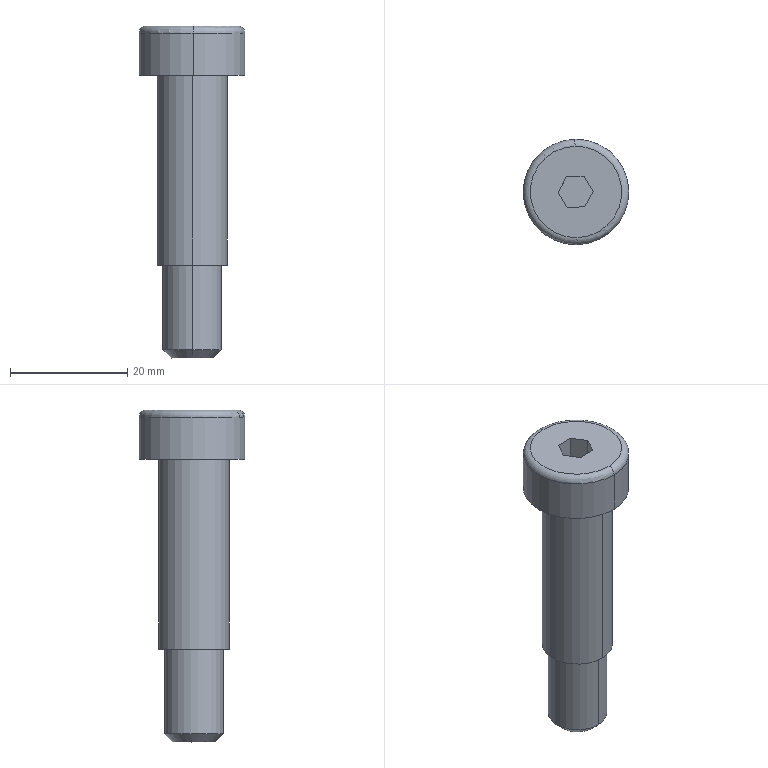Part | SolidWorks | features BaseBody 1 | 1 solid | 21 faces | box 18.001 x 18 x 56.624 mm | volume 6859 mm3 | plane 11 | cylinder 6 | torus 2 | cone 2 | commonest cylinder face diameters 10 x2 12 x2 18 x2
STEP:
#1=CARTESIAN_POINT('',(377.104,200.564,27.671));
#2=VERTEX_POINT('',#1);
#3=CARTESIAN_POINT('',(377.483,182.568,27.671));
#4=VERTEX_POINT('',#3);
#5=CARTESIAN_POINT('',(377.294,191.566,27.671));
#6=DIRECTION('',(-0.0001435,-0.000000521,1.));
#7=DIRECTION('',(0.02104,-0.9998,0.000002497));
#8=AXIS2_PLACEMENT_3D('',#5,#6,#7);
#9=CIRCLE('',#8,9.);
#10=EDGE_CURVE('',#2,#4,#9,.T.);
#11=ORIENTED_EDGE('',*,*,#10,.T.);
#12=CARTESIAN_POINT('',(377.458,183.768,28.871));
#13=VERTEX_POINT('',#12);
#14=CARTESIAN_POINT('',(377.458,183.768,27.671));
#15=DIRECTION('',(-0.9998,-0.02104,-0.0001435));
#16=DIRECTION('',(0.02104,-0.9998,0.));
#17=AXIS2_PLACEMENT_3D('',#14,#15,#16);
#18=CIRCLE('',#17,1.2);
#19=EDGE_CURVE('',#4,#13,#18,.T.);
#20=ORIENTED_EDGE('',*,*,#19,.T.);
#21=CARTESIAN_POINT('',(377.129,199.364,28.871));
#22=VERTEX_POINT('',#21);
#23=CARTESIAN_POINT('',(377.294,191.566,28.871));
#24=DIRECTION('',(-0.0001435,-0.000000521,1.));
#25=DIRECTION('',(0.02104,-0.9998,0.000002497));
#26=AXIS2_PLACEMENT_3D('',#23,#24,#25);
#27=CIRCLE('',#26,7.8);
#28=EDGE_CURVE('',#22,#13,#27,.T.);
#29=ORIENTED_EDGE('',*,*,#28,.F.);
#30=CARTESIAN_POINT('',(377.13,199.364,27.671));
#31=DIRECTION('',(0.9998,0.02104,0.0001435));
#32=DIRECTION('',(-0.02104,0.9998,0.));
#33=AXIS2_PLACEMENT_3D('',#30,#31,#32);
#34=CIRCLE('',#33,1.2);
#35=EDGE_CURVE('',#2,#22,#34,.T.);
#36=ORIENTED_EDGE('',*,*,#35,.F.);
#37=EDGE_LOOP('',(#11,#20,#29,#36));
#38=FACE_OUTER_BOUND('',#37,.T.);
#39=CARTESIAN_POINT('',(377.294,191.566,27.671));
#40=DIRECTION('',(-0.0001435,-0.000000521,1.));
#41=DIRECTION('',(-0.02104,0.9998,-0.000002497));
#42=AXIS2_PLACEMENT_3D('',#39,#40,#41);
#43=TOROIDAL_SURFACE('',#42,7.8,1.2);
#44=ADVANCED_FACE('',(#38),#43,.T.);
#45=CARTESIAN_POINT('',(377.484,182.568,20.471));
#46=VERTEX_POINT('',#45);
#47=CARTESIAN_POINT('',(377.105,200.564,20.471));
#48=VERTEX_POINT('',#47);
#49=CARTESIAN_POINT('',(377.295,191.566,20.471));
#50=DIRECTION('',(0.0001435,0.000000521,-1.));
#51=DIRECTION('',(-0.02104,0.9998,-0.000002497));
#52=AXIS2_PLACEMENT_3D('',#49,#50,#51);
#53=CIRCLE('',#52,9.);
#54=EDGE_CURVE('',#46,#48,#53,.T.);
#55=ORIENTED_EDGE('',*,*,#54,.F.);
#56=CARTESIAN_POINT('',(377.484,182.568,20.471));
#57=DIRECTION('',(-0.0001435,-0.000000521,1.));
#58=VECTOR('',#57,1000.);
#59=LINE('',#56,#58);
#60=EDGE_CURVE('',#46,#4,#59,.T.);
#61=ORIENTED_EDGE('',*,*,#60,.T.);
#62=ORIENTED_EDGE('',*,*,#10,.F.);
#63=CARTESIAN_POINT('',(377.105,200.564,20.471));
#64=DIRECTION('',(-0.0001435,-0.000000521,1.));
#65=VECTOR('',#64,1000.);
#66=LINE('',#63,#65);
#67=EDGE_CURVE('',#48,#2,#66,.T.);
#68=ORIENTED_EDGE('',*,*,#67,.F.);
#69=EDGE_LOOP('',(#55,#61,#62,#68));
#70=FACE_OUTER_BOUND('',#69,.T.);
#71=CARTESIAN_POINT('',(377.295,191.566,20.471));
#72=DIRECTION('',(-0.0001435,-0.000000521,1.));
#73=DIRECTION('',(-0.02104,0.9998,-0.000002497));
#74=AXIS2_PLACEMENT_3D('',#71,#72,#73);
#75=CYLINDRICAL_SURFACE('',#74,9.);
#76=ADVANCED_FACE('',(#70),#75,.T.);
#77=CARTESIAN_POINT('',(377.179,197.227,20.471));
#78=VERTEX_POINT('',#77);
#79=CARTESIAN_POINT('',(377.431,185.23,20.471));
#80=VERTEX_POINT('',#79);
#81=CARTESIAN_POINT('',(377.305,191.228,20.471));
#82=DIRECTION('',(-0.0001435,-0.000000521,1.));
#83=DIRECTION('',(0.02104,-0.9998,0.000002497));
#84=AXIS2_PLACEMENT_3D('',#81,#82,#83);
#85=CIRCLE('',#84,6.);
#86=EDGE_CURVE('',#78,#80,#85,.T.);
#87=ORIENTED_EDGE('',*,*,#86,.F.);
#88=CARTESIAN_POINT('',(377.183,197.227,-11.912));
#89=VERTEX_POINT('',#88);
#90=CARTESIAN_POINT('',(377.183,197.227,-11.726));
#91=DIRECTION('',(0.0001435,0.000000521,-1.));
#92=VECTOR('',#91,1000.);
#93=LINE('',#90,#92);
#94=EDGE_CURVE('',#78,#89,#93,.T.);
#95=ORIENTED_EDGE('',*,*,#94,.T.);
#96=CARTESIAN_POINT('',(377.436,185.23,-11.911));
#97=VERTEX_POINT('',#96);
#98=CARTESIAN_POINT('',(377.31,191.228,-11.911));
#99=DIRECTION('',(0.0001435,0.000000521,-1.));
#100=DIRECTION('',(-1.,0.,-0.0001435));
#101=AXIS2_PLACEMENT_3D('',#98,#99,#100);
#102=CIRCLE('',#101,6.);
#103=EDGE_CURVE('',#97,#89,#102,.T.);
#104=ORIENTED_EDGE('',*,*,#103,.F.);
#105=CARTESIAN_POINT('',(377.436,185.23,-11.726));
#106=DIRECTION('',(0.0001435,0.000000521,-1.));
#107=VECTOR('',#106,1000.);
#108=LINE('',#105,#107);
#109=EDGE_CURVE('',#80,#97,#108,.T.);
#110=ORIENTED_EDGE('',*,*,#109,.F.);
#111=EDGE_LOOP('',(#87,#95,#104,#110));
#112=FACE_OUTER_BOUND('',#111,.T.);
#113=CARTESIAN_POINT('',(377.309,191.228,-11.726));
#114=DIRECTION('',(0.0001435,0.000000521,-1.));
#115=DIRECTION('',(0.02104,-0.9998,0.000002497));
#116=AXIS2_PLACEMENT_3D('',#113,#114,#115);
#117=CYLINDRICAL_SURFACE('',#116,6.);
#118=ADVANCED_FACE('',(#112),#117,.T.);
#119=CARTESIAN_POINT('',(377.207,196.227,-11.912));
#120=VERTEX_POINT('',#119);
#121=CARTESIAN_POINT('',(377.417,186.23,-11.911));
#122=VERTEX_POINT('',#121);
#123=CARTESIAN_POINT('',(377.312,191.228,-11.911));
#124=DIRECTION('',(-0.0001435,-0.000000521,1.));
#125=DIRECTION('',(0.02104,-0.9998,0.000002497));
#126=AXIS2_PLACEMENT_3D('',#123,#124,#125);
#127=CIRCLE('',#126,5.);
#128=EDGE_CURVE('',#120,#122,#127,.T.);
#129=ORIENTED_EDGE('',*,*,#128,.F.);
#130=CARTESIAN_POINT('',(377.209,196.227,-26.352));
#131=VERTEX_POINT('',#130);
#132=CARTESIAN_POINT('',(377.207,196.227,-14.312));
#133=DIRECTION('',(0.0001435,0.000000521,-1.));
#134=VECTOR('',#133,1000.);
#135=LINE('',#132,#134);
#136=EDGE_CURVE('',#120,#131,#135,.T.);
#137=ORIENTED_EDGE('',*,*,#136,.T.);
#138=CARTESIAN_POINT('',(377.419,186.23,-26.351));
#139=VERTEX_POINT('',#138);
#140=CARTESIAN_POINT('',(377.314,191.228,-26.351));
#141=DIRECTION('',(0.0001435,0.000000521,-1.));
#142=DIRECTION('',(0.02104,-0.9998,0.000002497));
#143=AXIS2_PLACEMENT_3D('',#140,#141,#142);
#144=CIRCLE('',#143,5.);
#145=EDGE_CURVE('',#139,#131,#144,.T.);
#146=ORIENTED_EDGE('',*,*,#145,.F.);
#147=CARTESIAN_POINT('',(377.418,186.23,-14.311));
#148=DIRECTION('',(0.0001435,0.000000521,-1.));
#149=VECTOR('',#148,1000.);
#150=LINE('',#147,#149);
#151=EDGE_CURVE('',#122,#139,#150,.T.);
#152=ORIENTED_EDGE('',*,*,#151,.F.);
#153=EDGE_LOOP('',(#129,#137,#146,#152));
#154=FACE_OUTER_BOUND('',#153,.T.);
#155=CARTESIAN_POINT('',(377.312,191.228,-14.311));
#156=DIRECTION('',(0.0001435,0.000000521,-1.));
#157=DIRECTION('',(0.02104,-0.9998,0.000002497));
#158=AXIS2_PLACEMENT_3D('',#155,#156,#157);
#159=CYLINDRICAL_SURFACE('',#158,5.);
#160=ADVANCED_FACE('',(#154),#159,.T.);
#161=CARTESIAN_POINT('',(377.39,187.629,-27.751));
#162=VERTEX_POINT('',#161);
#163=CARTESIAN_POINT('',(377.239,194.828,-27.751));
#164=VERTEX_POINT('',#163);
#165=CARTESIAN_POINT('',(377.314,191.228,-27.751));
#166=DIRECTION('',(0.0001435,0.000000521,-1.));
#167=DIRECTION('',(0.02104,-0.9998,0.000002497));
#168=AXIS2_PLACEMENT_3D('',#165,#166,#167);
#169=CIRCLE('',#168,3.6);
#170=EDGE_CURVE('',#162,#164,#169,.T.);
#171=ORIENTED_EDGE('',*,*,#170,.F.);
#172=CARTESIAN_POINT('',(377.405,186.929,-27.051));
#173=DIRECTION('',(0.01477,-0.707,0.7071));
#174=VECTOR('',#173,1000.);
#175=LINE('',#172,#174);
#176=EDGE_CURVE('',#162,#139,#175,.T.);
#177=ORIENTED_EDGE('',*,*,#176,.T.);
#178=ORIENTED_EDGE('',*,*,#145,.T.);
#179=CARTESIAN_POINT('',(377.224,195.528,-27.052));
#180=DIRECTION('',(-0.01498,0.7069,0.7071));
#181=VECTOR('',#180,1000.);
#182=LINE('',#179,#181);
#183=EDGE_CURVE('',#164,#131,#182,.T.);
#184=ORIENTED_EDGE('',*,*,#183,.F.);
#185=EDGE_LOOP('',(#171,#177,#178,#184));
#186=FACE_OUTER_BOUND('',#185,.T.);
#187=CARTESIAN_POINT('',(377.314,191.228,-27.051));
#188=DIRECTION('',(-0.0001435,-0.000000521,1.));
#189=DIRECTION('',(-0.02104,0.9998,-0.000002497));
#190=AXIS2_PLACEMENT_3D('',#187,#188,#189);
#191=CONICAL_SURFACE('',#190,4.3,0.7854);
#192=ADVANCED_FACE('',(#186),#191,.T.);
#193=CARTESIAN_POINT('',(377.314,191.228,-27.751));
#194=DIRECTION('',(0.0001435,0.000000521,-1.));
#195=DIRECTION('',(0.02104,-0.9998,0.000002497));
#196=AXIS2_PLACEMENT_3D('',#193,#194,#195);
#197=CIRCLE('',#196,3.6);
#198=EDGE_CURVE('',#164,#162,#197,.T.);
#199=ORIENTED_EDGE('',*,*,#198,.T.);
#200=ORIENTED_EDGE('',*,*,#170,.T.);
#201=EDGE_LOOP('',(#199,#200));
#202=FACE_OUTER_BOUND('',#201,.T.);
#203=CARTESIAN_POINT('',(377.314,191.228,-27.751));
#204=DIRECTION('',(0.0001435,0.000000521,-1.));
#205=DIRECTION('',(0.,-1.,-0.000000521));
#206=AXIS2_PLACEMENT_3D('',#203,#204,#205);
#207=PLANE('',#206);
#208=ADVANCED_FACE('',(#202),#207,.T.);
#209=ORIENTED_EDGE('',*,*,#176,.F.);
#210=ORIENTED_EDGE('',*,*,#198,.F.);
#211=ORIENTED_EDGE('',*,*,#183,.T.);
#212=CARTESIAN_POINT('',(377.314,191.228,-26.351));
#213=DIRECTION('',(0.0001435,0.000000521,-1.));
#214=DIRECTION('',(0.02104,-0.9998,0.000002497));
#215=AXIS2_PLACEMENT_3D('',#212,#213,#214);
#216=CIRCLE('',#215,5.);
#217=EDGE_CURVE('',#131,#139,#216,.T.);
#218=ORIENTED_EDGE('',*,*,#217,.T.);
#219=EDGE_LOOP('',(#209,#210,#211,#218));
#220=FACE_OUTER_BOUND('',#219,.T.);
#221=CARTESIAN_POINT('',(377.314,191.228,-27.051));
#222=DIRECTION('',(-0.0001435,-0.000000521,1.));
#223=DIRECTION('',(-0.02104,0.9998,-0.000002497));
#224=AXIS2_PLACEMENT_3D('',#221,#222,#223);
#225=CONICAL_SURFACE('',#224,4.3,0.7854);
#226=ADVANCED_FACE('',(#220),#225,.T.);
#227=ORIENTED_EDGE('',*,*,#136,.F.);
#228=CARTESIAN_POINT('',(377.312,191.228,-11.911));
#229=DIRECTION('',(-0.0001435,-0.000000521,1.));
#230=DIRECTION('',(0.02104,-0.9998,0.000002497));
#231=AXIS2_PLACEMENT_3D('',#228,#229,#230);
#232=CIRCLE('',#231,5.);
#233=EDGE_CURVE('',#122,#120,#232,.T.);
#234=ORIENTED_EDGE('',*,*,#233,.F.);
#235=ORIENTED_EDGE('',*,*,#151,.T.);
#236=ORIENTED_EDGE('',*,*,#217,.F.);
#237=EDGE_LOOP('',(#227,#234,#235,#236));
#238=FACE_OUTER_BOUND('',#237,.T.);
#239=CARTESIAN_POINT('',(377.312,191.228,-14.311));
#240=DIRECTION('',(0.0001435,0.000000521,-1.));
#241=DIRECTION('',(0.02104,-0.9998,0.000002497));
#242=AXIS2_PLACEMENT_3D('',#239,#240,#241);
#243=CYLINDRICAL_SURFACE('',#242,5.);
#244=ADVANCED_FACE('',(#238),#243,.T.);
#245=ORIENTED_EDGE('',*,*,#233,.T.);
#246=ORIENTED_EDGE('',*,*,#128,.T.);
#247=EDGE_LOOP('',(#245,#246));
#248=FACE_BOUND('',#247,.T.);
#249=ORIENTED_EDGE('',*,*,#103,.T.);
#250=CARTESIAN_POINT('',(377.31,191.228,-11.911));
#251=DIRECTION('',(0.0001435,0.000000521,-1.));
#252=DIRECTION('',(-1.,0.,-0.0001435));
#253=AXIS2_PLACEMENT_3D('',#250,#251,#252);
#254=CIRCLE('',#253,6.);
#255=EDGE_CURVE('',#89,#97,#254,.T.);
#256=ORIENTED_EDGE('',*,*,#255,.T.);
#257=EDGE_LOOP('',(#249,#256));
#258=FACE_OUTER_BOUND('',#257,.T.);
#259=CARTESIAN_POINT('',(377.312,191.228,-11.911));
#260=DIRECTION('',(0.0001435,0.000000521,-1.));
#261=DIRECTION('',(0.,-1.,-0.000000521));
#262=AXIS2_PLACEMENT_3D('',#259,#260,#261);
#263=PLANE('',#262);
#264=ADVANCED_FACE('',(#248,#258),#263,.T.);
#265=ORIENTED_EDGE('',*,*,#94,.F.);
#266=CARTESIAN_POINT('',(377.305,191.228,20.471));
#267=DIRECTION('',(-0.0001435,-0.000000521,1.));
#268=DIRECTION('',(0.02104,-0.9998,0.000002497));
#269=AXIS2_PLACEMENT_3D('',#266,#267,#268);
#270=CIRCLE('',#269,6.);
#271=EDGE_CURVE('',#80,#78,#270,.T.);
#272=ORIENTED_EDGE('',*,*,#271,.F.);
#273=ORIENTED_EDGE('',*,*,#109,.T.);
#274=ORIENTED_EDGE('',*,*,#255,.F.);
#275=EDGE_LOOP('',(#265,#272,#273,#274));
#276=FACE_OUTER_BOUND('',#275,.T.);
#277=CARTESIAN_POINT('',(377.309,191.228,-11.726));
#278=DIRECTION('',(0.0001435,0.000000521,-1.));
#279=DIRECTION('',(0.02104,-0.9998,0.000002497));
#280=AXIS2_PLACEMENT_3D('',#277,#278,#279);
#281=CYLINDRICAL_SURFACE('',#280,6.);
#282=ADVANCED_FACE('',(#276),#281,.T.);
#283=ORIENTED_EDGE('',*,*,#271,.T.);
#284=ORIENTED_EDGE('',*,*,#86,.T.);
#285=EDGE_LOOP('',(#283,#284));
#286=FACE_BOUND('',#285,.T.);
#287=CARTESIAN_POINT('',(377.295,191.566,20.471));
#288=DIRECTION('',(0.0001435,0.000000521,-1.));
#289=DIRECTION('',(-0.02104,0.9998,-0.000002497));
#290=AXIS2_PLACEMENT_3D('',#287,#288,#289);
#291=CIRCLE('',#290,9.);
#292=EDGE_CURVE('',#48,#46,#291,.T.);
#293=ORIENTED_EDGE('',*,*,#292,.T.);
#294=ORIENTED_EDGE('',*,*,#54,.T.);
#295=EDGE_LOOP('',(#293,#294));
#296=FACE_OUTER_BOUND('',#295,.T.);
#297=CARTESIAN_POINT('',(377.295,191.566,20.471));
#298=DIRECTION('',(0.0001435,0.000000521,-1.));
#299=DIRECTION('',(0.,-1.,-0.000000521));
#300=AXIS2_PLACEMENT_3D('',#297,#298,#299);
#301=PLANE('',#300);
#302=ADVANCED_FACE('',(#286,#296),#301,.T.);
#303=ORIENTED_EDGE('',*,*,#60,.F.);
#304=ORIENTED_EDGE('',*,*,#292,.F.);
#305=ORIENTED_EDGE('',*,*,#67,.T.);
#306=CARTESIAN_POINT('',(377.294,191.566,27.671));
#307=DIRECTION('',(-0.0001435,-0.000000521,1.));
#308=DIRECTION('',(0.02104,-0.9998,0.000002497));
#309=AXIS2_PLACEMENT_3D('',#306,#307,#308);
#310=CIRCLE('',#309,9.);
#311=EDGE_CURVE('',#4,#2,#310,.T.);
#312=ORIENTED_EDGE('',*,*,#311,.F.);
#313=EDGE_LOOP('',(#303,#304,#305,#312));
#314=FACE_OUTER_BOUND('',#313,.T.);
#315=CARTESIAN_POINT('',(377.295,191.566,20.471));
#316=DIRECTION('',(-0.0001435,-0.000000521,1.));
#317=DIRECTION('',(-0.02104,0.9998,-0.000002497));
#318=AXIS2_PLACEMENT_3D('',#315,#316,#317);
#319=CYLINDRICAL_SURFACE('',#318,9.);
#320=ADVANCED_FACE('',(#314),#319,.T.);
#321=ORIENTED_EDGE('',*,*,#19,.F.);
#322=ORIENTED_EDGE('',*,*,#311,.T.);
#323=ORIENTED_EDGE('',*,*,#35,.T.);
#324=CARTESIAN_POINT('',(377.294,191.566,28.871));
#325=DIRECTION('',(-0.0001435,-0.000000521,1.));
#326=DIRECTION('',(0.02104,-0.9998,0.000002497));
#327=AXIS2_PLACEMENT_3D('',#324,#325,#326);
#328=CIRCLE('',#327,7.8);
#329=EDGE_CURVE('',#13,#22,#328,.T.);
#330=ORIENTED_EDGE('',*,*,#329,.F.);
#331=EDGE_LOOP('',(#321,#322,#323,#330));
#332=FACE_OUTER_BOUND('',#331,.T.);
#333=CARTESIAN_POINT('',(377.294,191.566,27.671));
#334=DIRECTION('',(-0.0001435,-0.000000521,1.));
#335=DIRECTION('',(-0.02104,0.9998,-0.000002497));
#336=AXIS2_PLACEMENT_3D('',#333,#334,#335);
#337=TOROIDAL_SURFACE('',#336,7.8,1.2);
#338=ADVANCED_FACE('',(#332),#337,.T.);
#339=CARTESIAN_POINT('',(375.792,188.955,22.871));
#340=VERTEX_POINT('',#339);
#341=CARTESIAN_POINT('',(378.792,189.018,22.871));
#342=VERTEX_POINT('',#341);
#343=CARTESIAN_POINT('',(375.792,188.955,22.871));
#344=DIRECTION('',(0.9998,0.02104,0.0001435));
#345=VECTOR('',#344,1000.);
#346=LINE('',#343,#345);
#347=EDGE_CURVE('',#340,#342,#346,.T.);
#348=ORIENTED_EDGE('',*,*,#347,.T.);
#349=CARTESIAN_POINT('',(380.237,191.648,22.871));
#350=VERTEX_POINT('',#349);
#351=CARTESIAN_POINT('',(378.792,189.018,22.871));
#352=DIRECTION('',(0.4817,0.8764,0.00006956));
#353=VECTOR('',#352,1000.);
#354=LINE('',#351,#353);
#355=EDGE_CURVE('',#342,#350,#354,.T.);
#356=ORIENTED_EDGE('',*,*,#355,.T.);
#357=CARTESIAN_POINT('',(378.682,194.213,22.871));
#358=VERTEX_POINT('',#357);
#359=CARTESIAN_POINT('',(380.237,191.648,22.871));
#360=DIRECTION('',(-0.5181,0.8553,-0.00007389));
#361=VECTOR('',#360,1000.);
#362=LINE('',#359,#361);
#363=EDGE_CURVE('',#350,#358,#362,.T.);
#364=ORIENTED_EDGE('',*,*,#363,.T.);
#365=CARTESIAN_POINT('',(375.683,194.15,22.871));
#366=VERTEX_POINT('',#365);
#367=CARTESIAN_POINT('',(378.682,194.213,22.871));
#368=DIRECTION('',(-0.9998,-0.02104,-0.0001435));
#369=VECTOR('',#368,1000.);
#370=LINE('',#367,#369);
#371=EDGE_CURVE('',#358,#366,#370,.T.);
#372=ORIENTED_EDGE('',*,*,#371,.T.);
#373=CARTESIAN_POINT('',(374.238,191.521,22.87));
#374=VERTEX_POINT('',#373);
#375=CARTESIAN_POINT('',(375.683,194.15,22.871));
#376=DIRECTION('',(-0.4817,-0.8764,-0.00006956));
#377=VECTOR('',#376,1000.);
#378=LINE('',#375,#377);
#379=EDGE_CURVE('',#366,#374,#378,.T.);
#380=ORIENTED_EDGE('',*,*,#379,.T.);
#381=CARTESIAN_POINT('',(374.238,191.521,22.87));
#382=DIRECTION('',(0.5181,-0.8553,0.00007389));
#383=VECTOR('',#382,1000.);
#384=LINE('',#381,#383);
#385=EDGE_CURVE('',#374,#340,#384,.T.);
#386=ORIENTED_EDGE('',*,*,#385,.T.);
#387=EDGE_LOOP('',(#348,#356,#364,#372,#380,#386));
#388=FACE_OUTER_BOUND('',#387,.T.);
#389=CARTESIAN_POINT('',(376.682,220.659,22.871));
#390=DIRECTION('',(-0.0001435,-0.000000521,1.));
#391=DIRECTION('',(-0.003633,1.,0.));
#392=AXIS2_PLACEMENT_3D('',#389,#390,#391);
#393=PLANE('',#392);
#394=ADVANCED_FACE('',(#388),#393,.T.);
#395=CARTESIAN_POINT('',(378.791,189.018,28.871));
#396=VERTEX_POINT('',#395);
#397=CARTESIAN_POINT('',(378.791,189.018,28.871));
#398=DIRECTION('',(0.0001435,0.000000521,-1.));
#399=VECTOR('',#398,1000.);
#400=LINE('',#397,#399);
#401=EDGE_CURVE('',#396,#342,#400,.T.);
#402=ORIENTED_EDGE('',*,*,#401,.T.);
#403=ORIENTED_EDGE('',*,*,#347,.F.);
#404=CARTESIAN_POINT('',(375.791,188.955,28.871));
#405=VERTEX_POINT('',#404);
#406=CARTESIAN_POINT('',(375.791,188.955,28.871));
#407=DIRECTION('',(0.0001435,0.000000521,-1.));
#408=VECTOR('',#407,1000.);
#409=LINE('',#406,#408);
#410=EDGE_CURVE('',#405,#340,#409,.T.);
#411=ORIENTED_EDGE('',*,*,#410,.F.);
#412=CARTESIAN_POINT('',(378.791,189.018,28.871));
#413=DIRECTION('',(-0.9998,-0.02104,-0.0001435));
#414=VECTOR('',#413,1000.);
#415=LINE('',#412,#414);
#416=EDGE_CURVE('',#396,#405,#415,.T.);
#417=ORIENTED_EDGE('',*,*,#416,.F.);
#418=EDGE_LOOP('',(#402,#403,#411,#417));
#419=FACE_OUTER_BOUND('',#418,.T.);
#420=CARTESIAN_POINT('',(378.792,189.018,22.871));
#421=DIRECTION('',(0.02104,-0.9998,0.000002497));
#422=DIRECTION('',(0.,-0.000002498,-1.));
#423=AXIS2_PLACEMENT_3D('',#420,#421,#422);
#424=PLANE('',#423);
#425=ADVANCED_FACE('',(#419),#424,.F.);
#426=CARTESIAN_POINT('',(380.236,191.648,28.871));
#427=VERTEX_POINT('',#426);
#428=CARTESIAN_POINT('',(380.236,191.648,28.871));
#429=DIRECTION('',(0.0001435,0.000000521,-1.));
#430=VECTOR('',#429,1000.);
#431=LINE('',#428,#430);
#432=EDGE_CURVE('',#427,#350,#431,.T.);
#433=ORIENTED_EDGE('',*,*,#432,.T.);
#434=ORIENTED_EDGE('',*,*,#355,.F.);
#435=ORIENTED_EDGE('',*,*,#401,.F.);
#436=CARTESIAN_POINT('',(380.236,191.648,28.871));
#437=DIRECTION('',(-0.4817,-0.8764,-0.00006956));
#438=VECTOR('',#437,1000.);
#439=LINE('',#436,#438);
#440=EDGE_CURVE('',#427,#396,#439,.T.);
#441=ORIENTED_EDGE('',*,*,#440,.F.);
#442=EDGE_LOOP('',(#433,#434,#435,#441));
#443=FACE_OUTER_BOUND('',#442,.T.);
#444=CARTESIAN_POINT('',(380.237,191.648,22.871));
#445=DIRECTION('',(0.8764,-0.4817,0.0001255));
#446=DIRECTION('',(0.,-0.0002605,-1.));
#447=AXIS2_PLACEMENT_3D('',#444,#445,#446);
#448=PLANE('',#447);
#449=ADVANCED_FACE('',(#443),#448,.F.);
#450=CARTESIAN_POINT('',(378.681,194.213,28.871));
#451=VERTEX_POINT('',#450);
#452=CARTESIAN_POINT('',(378.681,194.213,28.871));
#453=DIRECTION('',(0.0001435,0.000000521,-1.));
#454=VECTOR('',#453,1000.);
#455=LINE('',#452,#454);
#456=EDGE_CURVE('',#451,#358,#455,.T.);
#457=ORIENTED_EDGE('',*,*,#456,.T.);
#458=ORIENTED_EDGE('',*,*,#363,.F.);
#459=ORIENTED_EDGE('',*,*,#432,.F.);
#460=CARTESIAN_POINT('',(378.681,194.213,28.871));
#461=DIRECTION('',(0.5181,-0.8553,0.00007389));
#462=VECTOR('',#461,1000.);
#463=LINE('',#460,#462);
#464=EDGE_CURVE('',#451,#427,#463,.T.);
#465=ORIENTED_EDGE('',*,*,#464,.F.);
#466=EDGE_LOOP('',(#457,#458,#459,#465));
#467=FACE_OUTER_BOUND('',#466,.T.);
#468=CARTESIAN_POINT('',(378.682,194.213,22.871));
#469=DIRECTION('',(0.8553,0.5181,0.000123));
#470=DIRECTION('',(0.,0.0002374,-1.));
#471=AXIS2_PLACEMENT_3D('',#468,#469,#470);
#472=PLANE('',#471);
#473=ADVANCED_FACE('',(#467),#472,.F.);
#474=CARTESIAN_POINT('',(375.682,194.15,28.871));
#475=VERTEX_POINT('',#474);
#476=CARTESIAN_POINT('',(375.682,194.15,28.871));
#477=DIRECTION('',(0.0001435,0.000000521,-1.));
#478=VECTOR('',#477,1000.);
#479=LINE('',#476,#478);
#480=EDGE_CURVE('',#475,#366,#479,.T.);
#481=ORIENTED_EDGE('',*,*,#480,.T.);
#482=ORIENTED_EDGE('',*,*,#371,.F.);
#483=ORIENTED_EDGE('',*,*,#456,.F.);
#484=CARTESIAN_POINT('',(375.682,194.15,28.871));
#485=DIRECTION('',(0.9998,0.02104,0.0001435));
#486=VECTOR('',#485,1000.);
#487=LINE('',#484,#486);
#488=EDGE_CURVE('',#475,#451,#487,.T.);
#489=ORIENTED_EDGE('',*,*,#488,.F.);
#490=EDGE_LOOP('',(#481,#482,#483,#489));
#491=FACE_OUTER_BOUND('',#490,.T.);
#492=CARTESIAN_POINT('',(375.683,194.15,22.871));
#493=DIRECTION('',(-0.02104,0.9998,-0.000002497));
#494=DIRECTION('',(-0.0001187,0.,1.));
#495=AXIS2_PLACEMENT_3D('',#492,#493,#494);
#496=PLANE('',#495);
#497=ADVANCED_FACE('',(#491),#496,.F.);
#498=CARTESIAN_POINT('',(374.237,191.521,28.87));
#499=VERTEX_POINT('',#498);
#500=CARTESIAN_POINT('',(374.237,191.521,28.87));
#501=DIRECTION('',(0.0001435,0.000000521,-1.));
#502=VECTOR('',#501,1000.);
#503=LINE('',#500,#502);
#504=EDGE_CURVE('',#499,#374,#503,.T.);
#505=ORIENTED_EDGE('',*,*,#504,.T.);
#506=ORIENTED_EDGE('',*,*,#379,.F.);
#507=ORIENTED_EDGE('',*,*,#480,.F.);
#508=CARTESIAN_POINT('',(374.237,191.521,28.87));
#509=DIRECTION('',(0.4817,0.8764,0.00006956));
#510=VECTOR('',#509,1000.);
#511=LINE('',#508,#510);
#512=EDGE_CURVE('',#499,#475,#511,.T.);
#513=ORIENTED_EDGE('',*,*,#512,.F.);
#514=EDGE_LOOP('',(#505,#506,#507,#513));
#515=FACE_OUTER_BOUND('',#514,.T.);
#516=CARTESIAN_POINT('',(374.238,191.521,22.87));
#517=DIRECTION('',(-0.8764,0.4817,-0.0001255));
#518=DIRECTION('',(-0.0001432,0.,1.));
#519=AXIS2_PLACEMENT_3D('',#516,#517,#518);
#520=PLANE('',#519);
#521=ADVANCED_FACE('',(#515),#520,.F.);
#522=ORIENTED_EDGE('',*,*,#410,.T.);
#523=ORIENTED_EDGE('',*,*,#385,.F.);
#524=ORIENTED_EDGE('',*,*,#504,.F.);
#525=CARTESIAN_POINT('',(375.791,188.955,28.871));
#526=DIRECTION('',(-0.5181,0.8553,-0.00007389));
#527=VECTOR('',#526,1000.);
#528=LINE('',#525,#527);
#529=EDGE_CURVE('',#405,#499,#528,.T.);
#530=ORIENTED_EDGE('',*,*,#529,.F.);
#531=EDGE_LOOP('',(#522,#523,#524,#530));
#532=FACE_OUTER_BOUND('',#531,.T.);
#533=CARTESIAN_POINT('',(375.792,188.955,22.871));
#534=DIRECTION('',(-0.8553,-0.5181,-0.000123));
#535=DIRECTION('',(-0.5181,0.8553,0.));
#536=AXIS2_PLACEMENT_3D('',#533,#534,#535);
#537=PLANE('',#536);
#538=ADVANCED_FACE('',(#532),#537,.F.);
#539=ORIENTED_EDGE('',*,*,#512,.T.);
#540=ORIENTED_EDGE('',*,*,#488,.T.);
#541=ORIENTED_EDGE('',*,*,#464,.T.);
#542=ORIENTED_EDGE('',*,*,#440,.T.);
#543=ORIENTED_EDGE('',*,*,#416,.T.);
#544=ORIENTED_EDGE('',*,*,#529,.T.);
#545=EDGE_LOOP('',(#539,#540,#541,#542,#543,#544));
#546=FACE_BOUND('',#545,.T.);
#547=ORIENTED_EDGE('',*,*,#28,.T.);
#548=ORIENTED_EDGE('',*,*,#329,.T.);
#549=EDGE_LOOP('',(#547,#548));
#550=FACE_OUTER_BOUND('',#549,.T.);
#551=CARTESIAN_POINT('',(377.294,191.566,28.871));
#552=DIRECTION('',(-0.0001435,-0.000000521,1.));
#553=DIRECTION('',(-0.003633,1.,0.));
#554=AXIS2_PLACEMENT_3D('',#551,#552,#553);
#555=PLANE('',#554);
#556=ADVANCED_FACE('',(#546,#550),#555,.T.);
#557=CLOSED_SHELL('',(#44,#76,#118,#160,#192,#208,#226,#244,#264,#282,#302,#320,#338,#394,#425,#449,#473,#497,#521,#538,#556));
#558=MANIFOLD_SOLID_BREP('',#557);
#559=CARTESIAN_POINT('',(0.,0.,0.));
#560=DIRECTION('',(0.,0.,1.));
#561=DIRECTION('',(1.,0.,0.));
#562=AXIS2_PLACEMENT_3D('',#559,#560,#561);
#563=(LENGTH_UNIT()NAMED_UNIT(*)SI_UNIT(.MILLI.,.METRE.));
#564=UNCERTAINTY_MEASURE_WITH_UNIT(LENGTH_MEASURE(0.00001),#563,'','');
#565=(NAMED_UNIT(*)PLANE_ANGLE_UNIT()SI_UNIT($,.RADIAN.));
#566=(NAMED_UNIT(*)SI_UNIT($,.STERADIAN.)SOLID_ANGLE_UNIT());
#567=(GEOMETRIC_REPRESENTATION_CONTEXT(3)GLOBAL_UNCERTAINTY_ASSIGNED_CONTEXT((#564))GLOBAL_UNIT_ASSIGNED_CONTEXT((#563,#565,#566))REPRESENTATION_CONTEXT('',''));
#568=ADVANCED_BREP_SHAPE_REPRESENTATION('',(#558,#562),#567);